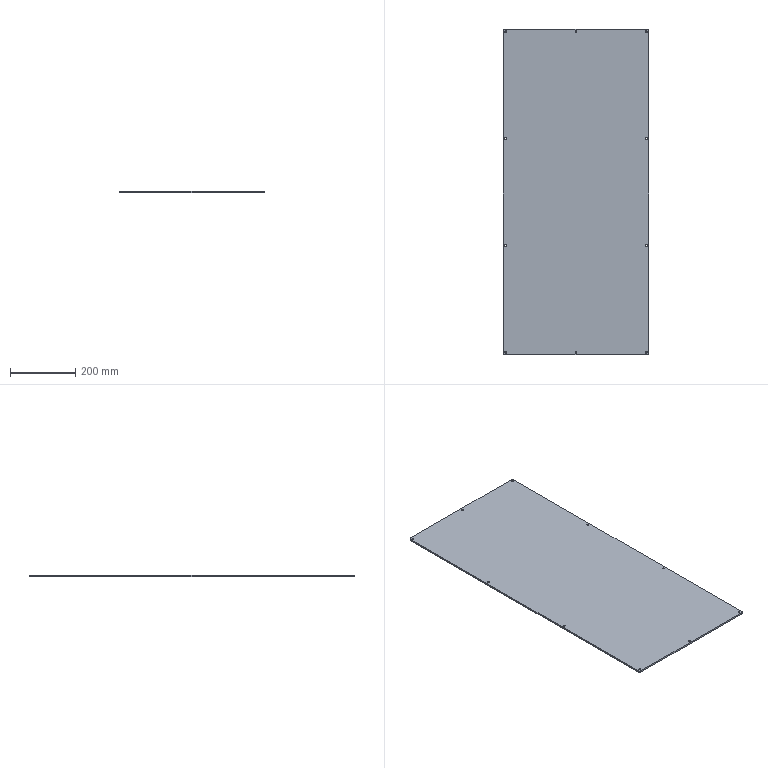Part | NX | features BREP 1 | 1 solid | 30 faces | box 446 x 996 x 5 mm | volume 2219652 mm3 | cylinder 24 | plane 6 | commonest cylinder face diameters 5.8 x20 10 x4
STEP:
#1=CARTESIAN_POINT('',(-218.,498.,5.));
#2=VERTEX_POINT('',#1);
#3=CARTESIAN_POINT('',(-223.,493.,5.));
#4=VERTEX_POINT('',#3);
#5=CARTESIAN_POINT('',(-218.,493.,5.));
#6=DIRECTION('',(0.,0.,1.));
#7=DIRECTION('',(1.,0.,0.));
#8=AXIS2_PLACEMENT_3D('',#5,#6,#7);
#9=CIRCLE('',#8,5.);
#10=EDGE_CURVE('',#2,#4,#9,.T.);
#11=ORIENTED_EDGE('',*,*,#10,.F.);
#12=CARTESIAN_POINT('',(-218.,498.,0.));
#13=VERTEX_POINT('',#12);
#14=CARTESIAN_POINT('',(-218.,498.,5.));
#15=DIRECTION('',(0.,0.,1.));
#16=VECTOR('',#15,1000.);
#17=LINE('',#14,#16);
#18=EDGE_CURVE('',#13,#2,#17,.T.);
#19=ORIENTED_EDGE('',*,*,#18,.F.);
#20=CARTESIAN_POINT('',(-223.,493.,0.));
#21=VERTEX_POINT('',#20);
#22=CARTESIAN_POINT('',(-218.,493.,0.));
#23=DIRECTION('',(0.,0.,-1.));
#24=DIRECTION('',(1.,0.,0.));
#25=AXIS2_PLACEMENT_3D('',#22,#23,#24);
#26=CIRCLE('',#25,5.);
#27=EDGE_CURVE('',#21,#13,#26,.T.);
#28=ORIENTED_EDGE('',*,*,#27,.F.);
#29=CARTESIAN_POINT('',(-223.,493.,5.));
#30=DIRECTION('',(0.,0.,-1.));
#31=VECTOR('',#30,1000.);
#32=LINE('',#29,#31);
#33=EDGE_CURVE('',#4,#21,#32,.T.);
#34=ORIENTED_EDGE('',*,*,#33,.F.);
#35=EDGE_LOOP('',(#11,#19,#28,#34));
#36=FACE_BOUND('',#35,.T.);
#37=CARTESIAN_POINT('',(-218.,493.,5.));
#38=DIRECTION('',(0.,0.,-1.));
#39=DIRECTION('',(-1.,0.,0.));
#40=AXIS2_PLACEMENT_3D('',#37,#38,#39);
#41=CYLINDRICAL_SURFACE('',#40,5.);
#42=ADVANCED_FACE('',(#36),#41,.T.);
#43=CARTESIAN_POINT('',(223.,493.,5.));
#44=VERTEX_POINT('',#43);
#45=CARTESIAN_POINT('',(218.,498.,5.));
#46=VERTEX_POINT('',#45);
#47=CARTESIAN_POINT('',(218.,493.,5.));
#48=DIRECTION('',(0.,0.,1.));
#49=DIRECTION('',(1.,0.,0.));
#50=AXIS2_PLACEMENT_3D('',#47,#48,#49);
#51=CIRCLE('',#50,5.);
#52=EDGE_CURVE('',#44,#46,#51,.T.);
#53=ORIENTED_EDGE('',*,*,#52,.F.);
#54=CARTESIAN_POINT('',(223.,493.,0.));
#55=VERTEX_POINT('',#54);
#56=CARTESIAN_POINT('',(223.,493.,5.));
#57=DIRECTION('',(0.,0.,1.));
#58=VECTOR('',#57,1000.);
#59=LINE('',#56,#58);
#60=EDGE_CURVE('',#55,#44,#59,.T.);
#61=ORIENTED_EDGE('',*,*,#60,.F.);
#62=CARTESIAN_POINT('',(218.,498.,0.));
#63=VERTEX_POINT('',#62);
#64=CARTESIAN_POINT('',(218.,493.,0.));
#65=DIRECTION('',(0.,0.,-1.));
#66=DIRECTION('',(1.,0.,0.));
#67=AXIS2_PLACEMENT_3D('',#64,#65,#66);
#68=CIRCLE('',#67,5.);
#69=EDGE_CURVE('',#63,#55,#68,.T.);
#70=ORIENTED_EDGE('',*,*,#69,.F.);
#71=CARTESIAN_POINT('',(218.,498.,5.));
#72=DIRECTION('',(0.,0.,-1.));
#73=VECTOR('',#72,1000.);
#74=LINE('',#71,#73);
#75=EDGE_CURVE('',#46,#63,#74,.T.);
#76=ORIENTED_EDGE('',*,*,#75,.F.);
#77=EDGE_LOOP('',(#53,#61,#70,#76));
#78=FACE_BOUND('',#77,.T.);
#79=CARTESIAN_POINT('',(218.,493.,5.));
#80=DIRECTION('',(0.,0.,-1.));
#81=DIRECTION('',(-1.,0.,0.));
#82=AXIS2_PLACEMENT_3D('',#79,#80,#81);
#83=CYLINDRICAL_SURFACE('',#82,5.);
#84=ADVANCED_FACE('',(#78),#83,.T.);
#85=CARTESIAN_POINT('',(218.,-498.,5.));
#86=VERTEX_POINT('',#85);
#87=CARTESIAN_POINT('',(223.,-493.,5.));
#88=VERTEX_POINT('',#87);
#89=CARTESIAN_POINT('',(218.,-493.,5.));
#90=DIRECTION('',(0.,0.,1.));
#91=DIRECTION('',(1.,0.,0.));
#92=AXIS2_PLACEMENT_3D('',#89,#90,#91);
#93=CIRCLE('',#92,5.);
#94=EDGE_CURVE('',#86,#88,#93,.T.);
#95=ORIENTED_EDGE('',*,*,#94,.F.);
#96=CARTESIAN_POINT('',(218.,-498.,0.));
#97=VERTEX_POINT('',#96);
#98=CARTESIAN_POINT('',(218.,-498.,5.));
#99=DIRECTION('',(0.,0.,1.));
#100=VECTOR('',#99,1000.);
#101=LINE('',#98,#100);
#102=EDGE_CURVE('',#97,#86,#101,.T.);
#103=ORIENTED_EDGE('',*,*,#102,.F.);
#104=CARTESIAN_POINT('',(223.,-493.,0.));
#105=VERTEX_POINT('',#104);
#106=CARTESIAN_POINT('',(218.,-493.,0.));
#107=DIRECTION('',(0.,0.,-1.));
#108=DIRECTION('',(1.,0.,0.));
#109=AXIS2_PLACEMENT_3D('',#106,#107,#108);
#110=CIRCLE('',#109,5.);
#111=EDGE_CURVE('',#105,#97,#110,.T.);
#112=ORIENTED_EDGE('',*,*,#111,.F.);
#113=CARTESIAN_POINT('',(223.,-493.,5.));
#114=DIRECTION('',(0.,0.,-1.));
#115=VECTOR('',#114,1000.);
#116=LINE('',#113,#115);
#117=EDGE_CURVE('',#88,#105,#116,.T.);
#118=ORIENTED_EDGE('',*,*,#117,.F.);
#119=EDGE_LOOP('',(#95,#103,#112,#118));
#120=FACE_BOUND('',#119,.T.);
#121=CARTESIAN_POINT('',(218.,-493.,5.));
#122=DIRECTION('',(0.,0.,-1.));
#123=DIRECTION('',(-1.,0.,0.));
#124=AXIS2_PLACEMENT_3D('',#121,#122,#123);
#125=CYLINDRICAL_SURFACE('',#124,5.);
#126=ADVANCED_FACE('',(#120),#125,.T.);
#127=CARTESIAN_POINT('',(-223.,-493.,5.));
#128=VERTEX_POINT('',#127);
#129=CARTESIAN_POINT('',(-218.,-498.,5.));
#130=VERTEX_POINT('',#129);
#131=CARTESIAN_POINT('',(-218.,-493.,5.));
#132=DIRECTION('',(0.,0.,1.));
#133=DIRECTION('',(1.,0.,0.));
#134=AXIS2_PLACEMENT_3D('',#131,#132,#133);
#135=CIRCLE('',#134,5.);
#136=EDGE_CURVE('',#128,#130,#135,.T.);
#137=ORIENTED_EDGE('',*,*,#136,.F.);
#138=CARTESIAN_POINT('',(-223.,-493.,0.));
#139=VERTEX_POINT('',#138);
#140=CARTESIAN_POINT('',(-223.,-493.,5.));
#141=DIRECTION('',(0.,0.,1.));
#142=VECTOR('',#141,1000.);
#143=LINE('',#140,#142);
#144=EDGE_CURVE('',#139,#128,#143,.T.);
#145=ORIENTED_EDGE('',*,*,#144,.F.);
#146=CARTESIAN_POINT('',(-218.,-498.,0.));
#147=VERTEX_POINT('',#146);
#148=CARTESIAN_POINT('',(-218.,-493.,0.));
#149=DIRECTION('',(0.,0.,-1.));
#150=DIRECTION('',(1.,0.,0.));
#151=AXIS2_PLACEMENT_3D('',#148,#149,#150);
#152=CIRCLE('',#151,5.);
#153=EDGE_CURVE('',#147,#139,#152,.T.);
#154=ORIENTED_EDGE('',*,*,#153,.F.);
#155=CARTESIAN_POINT('',(-218.,-498.,5.));
#156=DIRECTION('',(0.,0.,-1.));
#157=VECTOR('',#156,1000.);
#158=LINE('',#155,#157);
#159=EDGE_CURVE('',#130,#147,#158,.T.);
#160=ORIENTED_EDGE('',*,*,#159,.F.);
#161=EDGE_LOOP('',(#137,#145,#154,#160));
#162=FACE_BOUND('',#161,.T.);
#163=CARTESIAN_POINT('',(-218.,-493.,5.));
#164=DIRECTION('',(0.,0.,-1.));
#165=DIRECTION('',(-1.,0.,0.));
#166=AXIS2_PLACEMENT_3D('',#163,#164,#165);
#167=CYLINDRICAL_SURFACE('',#166,5.);
#168=ADVANCED_FACE('',(#162),#167,.T.);
#169=CARTESIAN_POINT('',(212.1,-490.,5.));
#170=VERTEX_POINT('',#169);
#171=CARTESIAN_POINT('',(212.1,-490.,0.));
#172=VERTEX_POINT('',#171);
#173=CARTESIAN_POINT('',(212.1,-490.,0.));
#174=DIRECTION('',(0.,0.,1.));
#175=VECTOR('',#174,1000.);
#176=LINE('',#173,#175);
#177=EDGE_CURVE('',#170,#172,#176,.F.);
#178=ORIENTED_EDGE('',*,*,#177,.T.);
#179=CARTESIAN_POINT('',(217.9,-490.,0.));
#180=VERTEX_POINT('',#179);
#181=CARTESIAN_POINT('',(215.,-490.,0.));
#182=DIRECTION('',(0.,0.,1.));
#183=DIRECTION('',(1.,0.,0.));
#184=AXIS2_PLACEMENT_3D('',#181,#182,#183);
#185=CIRCLE('',#184,2.9);
#186=EDGE_CURVE('',#180,#172,#185,.T.);
#187=ORIENTED_EDGE('',*,*,#186,.F.);
#188=CARTESIAN_POINT('',(217.9,-490.,5.));
#189=VERTEX_POINT('',#188);
#190=CARTESIAN_POINT('',(217.9,-490.,0.));
#191=DIRECTION('',(0.,0.,1.));
#192=VECTOR('',#191,1000.);
#193=LINE('',#190,#192);
#194=EDGE_CURVE('',#189,#180,#193,.F.);
#195=ORIENTED_EDGE('',*,*,#194,.F.);
#196=CARTESIAN_POINT('',(215.,-490.,5.));
#197=DIRECTION('',(0.,0.,1.));
#198=DIRECTION('',(1.,0.,0.));
#199=AXIS2_PLACEMENT_3D('',#196,#197,#198);
#200=CIRCLE('',#199,2.9);
#201=EDGE_CURVE('',#189,#170,#200,.T.);
#202=ORIENTED_EDGE('',*,*,#201,.T.);
#203=EDGE_LOOP('',(#178,#187,#195,#202));
#204=FACE_BOUND('',#203,.T.);
#205=CARTESIAN_POINT('',(215.,-490.,0.));
#206=DIRECTION('',(0.,0.,1.));
#207=DIRECTION('',(1.,0.,0.));
#208=AXIS2_PLACEMENT_3D('',#205,#206,#207);
#209=CYLINDRICAL_SURFACE('',#208,2.9);
#210=ADVANCED_FACE('',(#204),#209,.F.);
#211=CARTESIAN_POINT('',(212.1,163.333,5.));
#212=VERTEX_POINT('',#211);
#213=CARTESIAN_POINT('',(212.1,163.333,0.));
#214=VERTEX_POINT('',#213);
#215=CARTESIAN_POINT('',(212.1,163.333,0.));
#216=DIRECTION('',(0.,0.,1.));
#217=VECTOR('',#216,1000.);
#218=LINE('',#215,#217);
#219=EDGE_CURVE('',#212,#214,#218,.F.);
#220=ORIENTED_EDGE('',*,*,#219,.T.);
#221=CARTESIAN_POINT('',(217.9,163.333,0.));
#222=VERTEX_POINT('',#221);
#223=CARTESIAN_POINT('',(215.,163.333,0.));
#224=DIRECTION('',(0.,0.,1.));
#225=DIRECTION('',(1.,0.,0.));
#226=AXIS2_PLACEMENT_3D('',#223,#224,#225);
#227=CIRCLE('',#226,2.9);
#228=EDGE_CURVE('',#222,#214,#227,.T.);
#229=ORIENTED_EDGE('',*,*,#228,.F.);
#230=CARTESIAN_POINT('',(217.9,163.333,5.));
#231=VERTEX_POINT('',#230);
#232=CARTESIAN_POINT('',(217.9,163.333,0.));
#233=DIRECTION('',(0.,0.,1.));
#234=VECTOR('',#233,1000.);
#235=LINE('',#232,#234);
#236=EDGE_CURVE('',#231,#222,#235,.F.);
#237=ORIENTED_EDGE('',*,*,#236,.F.);
#238=CARTESIAN_POINT('',(215.,163.333,5.));
#239=DIRECTION('',(0.,0.,1.));
#240=DIRECTION('',(1.,0.,0.));
#241=AXIS2_PLACEMENT_3D('',#238,#239,#240);
#242=CIRCLE('',#241,2.9);
#243=EDGE_CURVE('',#231,#212,#242,.T.);
#244=ORIENTED_EDGE('',*,*,#243,.T.);
#245=EDGE_LOOP('',(#220,#229,#237,#244));
#246=FACE_BOUND('',#245,.T.);
#247=CARTESIAN_POINT('',(215.,163.333,0.));
#248=DIRECTION('',(0.,0.,1.));
#249=DIRECTION('',(1.,0.,0.));
#250=AXIS2_PLACEMENT_3D('',#247,#248,#249);
#251=CYLINDRICAL_SURFACE('',#250,2.9);
#252=ADVANCED_FACE('',(#246),#251,.F.);
#253=CARTESIAN_POINT('',(212.1,-163.333,5.));
#254=VERTEX_POINT('',#253);
#255=CARTESIAN_POINT('',(212.1,-163.333,0.));
#256=VERTEX_POINT('',#255);
#257=CARTESIAN_POINT('',(212.1,-163.333,0.));
#258=DIRECTION('',(0.,0.,1.));
#259=VECTOR('',#258,1000.);
#260=LINE('',#257,#259);
#261=EDGE_CURVE('',#254,#256,#260,.F.);
#262=ORIENTED_EDGE('',*,*,#261,.T.);
#263=CARTESIAN_POINT('',(217.9,-163.333,0.));
#264=VERTEX_POINT('',#263);
#265=CARTESIAN_POINT('',(215.,-163.333,0.));
#266=DIRECTION('',(0.,0.,1.));
#267=DIRECTION('',(1.,0.,0.));
#268=AXIS2_PLACEMENT_3D('',#265,#266,#267);
#269=CIRCLE('',#268,2.9);
#270=EDGE_CURVE('',#264,#256,#269,.T.);
#271=ORIENTED_EDGE('',*,*,#270,.F.);
#272=CARTESIAN_POINT('',(217.9,-163.333,5.));
#273=VERTEX_POINT('',#272);
#274=CARTESIAN_POINT('',(217.9,-163.333,0.));
#275=DIRECTION('',(0.,0.,1.));
#276=VECTOR('',#275,1000.);
#277=LINE('',#274,#276);
#278=EDGE_CURVE('',#273,#264,#277,.F.);
#279=ORIENTED_EDGE('',*,*,#278,.F.);
#280=CARTESIAN_POINT('',(215.,-163.333,5.));
#281=DIRECTION('',(0.,0.,1.));
#282=DIRECTION('',(1.,0.,0.));
#283=AXIS2_PLACEMENT_3D('',#280,#281,#282);
#284=CIRCLE('',#283,2.9);
#285=EDGE_CURVE('',#273,#254,#284,.T.);
#286=ORIENTED_EDGE('',*,*,#285,.T.);
#287=EDGE_LOOP('',(#262,#271,#279,#286));
#288=FACE_BOUND('',#287,.T.);
#289=CARTESIAN_POINT('',(215.,-163.333,0.));
#290=DIRECTION('',(0.,0.,1.));
#291=DIRECTION('',(1.,0.,0.));
#292=AXIS2_PLACEMENT_3D('',#289,#290,#291);
#293=CYLINDRICAL_SURFACE('',#292,2.9);
#294=ADVANCED_FACE('',(#288),#293,.F.);
#295=CARTESIAN_POINT('',(-217.9,163.333,5.));
#296=VERTEX_POINT('',#295);
#297=CARTESIAN_POINT('',(-217.9,163.333,0.));
#298=VERTEX_POINT('',#297);
#299=CARTESIAN_POINT('',(-217.9,163.333,0.));
#300=DIRECTION('',(0.,0.,1.));
#301=VECTOR('',#300,1000.);
#302=LINE('',#299,#301);
#303=EDGE_CURVE('',#296,#298,#302,.F.);
#304=ORIENTED_EDGE('',*,*,#303,.T.);
#305=CARTESIAN_POINT('',(-212.1,163.333,0.));
#306=VERTEX_POINT('',#305);
#307=CARTESIAN_POINT('',(-215.,163.333,0.));
#308=DIRECTION('',(0.,0.,1.));
#309=DIRECTION('',(1.,0.,0.));
#310=AXIS2_PLACEMENT_3D('',#307,#308,#309);
#311=CIRCLE('',#310,2.9);
#312=EDGE_CURVE('',#306,#298,#311,.T.);
#313=ORIENTED_EDGE('',*,*,#312,.F.);
#314=CARTESIAN_POINT('',(-212.1,163.333,5.));
#315=VERTEX_POINT('',#314);
#316=CARTESIAN_POINT('',(-212.1,163.333,0.));
#317=DIRECTION('',(0.,0.,1.));
#318=VECTOR('',#317,1000.);
#319=LINE('',#316,#318);
#320=EDGE_CURVE('',#315,#306,#319,.F.);
#321=ORIENTED_EDGE('',*,*,#320,.F.);
#322=CARTESIAN_POINT('',(-215.,163.333,5.));
#323=DIRECTION('',(0.,0.,1.));
#324=DIRECTION('',(1.,0.,0.));
#325=AXIS2_PLACEMENT_3D('',#322,#323,#324);
#326=CIRCLE('',#325,2.9);
#327=EDGE_CURVE('',#315,#296,#326,.T.);
#328=ORIENTED_EDGE('',*,*,#327,.T.);
#329=EDGE_LOOP('',(#304,#313,#321,#328));
#330=FACE_BOUND('',#329,.T.);
#331=CARTESIAN_POINT('',(-215.,163.333,0.));
#332=DIRECTION('',(0.,0.,1.));
#333=DIRECTION('',(1.,0.,0.));
#334=AXIS2_PLACEMENT_3D('',#331,#332,#333);
#335=CYLINDRICAL_SURFACE('',#334,2.9);
#336=ADVANCED_FACE('',(#330),#335,.F.);
#337=CARTESIAN_POINT('',(-2.9,-490.,5.));
#338=VERTEX_POINT('',#337);
#339=CARTESIAN_POINT('',(-2.9,-490.,0.));
#340=VERTEX_POINT('',#339);
#341=CARTESIAN_POINT('',(-2.9,-490.,0.));
#342=DIRECTION('',(0.,0.,1.));
#343=VECTOR('',#342,1000.);
#344=LINE('',#341,#343);
#345=EDGE_CURVE('',#338,#340,#344,.F.);
#346=ORIENTED_EDGE('',*,*,#345,.T.);
#347=CARTESIAN_POINT('',(2.9,-490.,0.));
#348=VERTEX_POINT('',#347);
#349=CARTESIAN_POINT('',(0.,-490.,0.));
#350=DIRECTION('',(0.,0.,1.));
#351=DIRECTION('',(1.,0.,0.));
#352=AXIS2_PLACEMENT_3D('',#349,#350,#351);
#353=CIRCLE('',#352,2.9);
#354=EDGE_CURVE('',#348,#340,#353,.T.);
#355=ORIENTED_EDGE('',*,*,#354,.F.);
#356=CARTESIAN_POINT('',(2.9,-490.,5.));
#357=VERTEX_POINT('',#356);
#358=CARTESIAN_POINT('',(2.9,-490.,0.));
#359=DIRECTION('',(0.,0.,1.));
#360=VECTOR('',#359,1000.);
#361=LINE('',#358,#360);
#362=EDGE_CURVE('',#357,#348,#361,.F.);
#363=ORIENTED_EDGE('',*,*,#362,.F.);
#364=CARTESIAN_POINT('',(0.,-490.,5.));
#365=DIRECTION('',(0.,0.,1.));
#366=DIRECTION('',(1.,0.,0.));
#367=AXIS2_PLACEMENT_3D('',#364,#365,#366);
#368=CIRCLE('',#367,2.9);
#369=EDGE_CURVE('',#357,#338,#368,.T.);
#370=ORIENTED_EDGE('',*,*,#369,.T.);
#371=EDGE_LOOP('',(#346,#355,#363,#370));
#372=FACE_BOUND('',#371,.T.);
#373=CARTESIAN_POINT('',(0.,-490.,0.));
#374=DIRECTION('',(0.,0.,1.));
#375=DIRECTION('',(1.,0.,0.));
#376=AXIS2_PLACEMENT_3D('',#373,#374,#375);
#377=CYLINDRICAL_SURFACE('',#376,2.9);
#378=ADVANCED_FACE('',(#372),#377,.F.);
#379=CARTESIAN_POINT('',(-217.9,-490.,5.));
#380=VERTEX_POINT('',#379);
#381=CARTESIAN_POINT('',(-217.9,-490.,0.));
#382=VERTEX_POINT('',#381);
#383=CARTESIAN_POINT('',(-217.9,-490.,0.));
#384=DIRECTION('',(0.,0.,1.));
#385=VECTOR('',#384,1000.);
#386=LINE('',#383,#385);
#387=EDGE_CURVE('',#380,#382,#386,.F.);
#388=ORIENTED_EDGE('',*,*,#387,.T.);
#389=CARTESIAN_POINT('',(-212.1,-490.,0.));
#390=VERTEX_POINT('',#389);
#391=CARTESIAN_POINT('',(-215.,-490.,0.));
#392=DIRECTION('',(0.,0.,1.));
#393=DIRECTION('',(1.,0.,0.));
#394=AXIS2_PLACEMENT_3D('',#391,#392,#393);
#395=CIRCLE('',#394,2.9);
#396=EDGE_CURVE('',#390,#382,#395,.T.);
#397=ORIENTED_EDGE('',*,*,#396,.F.);
#398=CARTESIAN_POINT('',(-212.1,-490.,5.));
#399=VERTEX_POINT('',#398);
#400=CARTESIAN_POINT('',(-212.1,-490.,0.));
#401=DIRECTION('',(0.,0.,1.));
#402=VECTOR('',#401,1000.);
#403=LINE('',#400,#402);
#404=EDGE_CURVE('',#399,#390,#403,.F.);
#405=ORIENTED_EDGE('',*,*,#404,.F.);
#406=CARTESIAN_POINT('',(-215.,-490.,5.));
#407=DIRECTION('',(0.,0.,1.));
#408=DIRECTION('',(1.,0.,0.));
#409=AXIS2_PLACEMENT_3D('',#406,#407,#408);
#410=CIRCLE('',#409,2.9);
#411=EDGE_CURVE('',#399,#380,#410,.T.);
#412=ORIENTED_EDGE('',*,*,#411,.T.);
#413=EDGE_LOOP('',(#388,#397,#405,#412));
#414=FACE_BOUND('',#413,.T.);
#415=CARTESIAN_POINT('',(-215.,-490.,0.));
#416=DIRECTION('',(0.,0.,1.));
#417=DIRECTION('',(1.,0.,0.));
#418=AXIS2_PLACEMENT_3D('',#415,#416,#417);
#419=CYLINDRICAL_SURFACE('',#418,2.9);
#420=ADVANCED_FACE('',(#414),#419,.F.);
#421=CARTESIAN_POINT('',(212.1,490.,5.));
#422=VERTEX_POINT('',#421);
#423=CARTESIAN_POINT('',(212.1,490.,0.));
#424=VERTEX_POINT('',#423);
#425=CARTESIAN_POINT('',(212.1,490.,0.));
#426=DIRECTION('',(0.,0.,1.));
#427=VECTOR('',#426,1000.);
#428=LINE('',#425,#427);
#429=EDGE_CURVE('',#422,#424,#428,.F.);
#430=ORIENTED_EDGE('',*,*,#429,.T.);
#431=CARTESIAN_POINT('',(217.9,490.,0.));
#432=VERTEX_POINT('',#431);
#433=CARTESIAN_POINT('',(215.,490.,0.));
#434=DIRECTION('',(0.,0.,1.));
#435=DIRECTION('',(1.,0.,0.));
#436=AXIS2_PLACEMENT_3D('',#433,#434,#435);
#437=CIRCLE('',#436,2.9);
#438=EDGE_CURVE('',#432,#424,#437,.T.);
#439=ORIENTED_EDGE('',*,*,#438,.F.);
#440=CARTESIAN_POINT('',(217.9,490.,5.));
#441=VERTEX_POINT('',#440);
#442=CARTESIAN_POINT('',(217.9,490.,0.));
#443=DIRECTION('',(0.,0.,1.));
#444=VECTOR('',#443,1000.);
#445=LINE('',#442,#444);
#446=EDGE_CURVE('',#441,#432,#445,.F.);
#447=ORIENTED_EDGE('',*,*,#446,.F.);
#448=CARTESIAN_POINT('',(215.,490.,5.));
#449=DIRECTION('',(0.,0.,1.));
#450=DIRECTION('',(1.,0.,0.));
#451=AXIS2_PLACEMENT_3D('',#448,#449,#450);
#452=CIRCLE('',#451,2.9);
#453=EDGE_CURVE('',#441,#422,#452,.T.);
#454=ORIENTED_EDGE('',*,*,#453,.T.);
#455=EDGE_LOOP('',(#430,#439,#447,#454));
#456=FACE_BOUND('',#455,.T.);
#457=CARTESIAN_POINT('',(215.,490.,0.));
#458=DIRECTION('',(0.,0.,1.));
#459=DIRECTION('',(1.,0.,0.));
#460=AXIS2_PLACEMENT_3D('',#457,#458,#459);
#461=CYLINDRICAL_SURFACE('',#460,2.9);
#462=ADVANCED_FACE('',(#456),#461,.F.);
#463=CARTESIAN_POINT('',(-2.9,490.,5.));
#464=VERTEX_POINT('',#463);
#465=CARTESIAN_POINT('',(-2.9,490.,0.));
#466=VERTEX_POINT('',#465);
#467=CARTESIAN_POINT('',(-2.9,490.,0.));
#468=DIRECTION('',(0.,0.,1.));
#469=VECTOR('',#468,1000.);
#470=LINE('',#467,#469);
#471=EDGE_CURVE('',#464,#466,#470,.F.);
#472=ORIENTED_EDGE('',*,*,#471,.T.);
#473=CARTESIAN_POINT('',(2.9,490.,0.));
#474=VERTEX_POINT('',#473);
#475=CARTESIAN_POINT('',(0.,490.,0.));
#476=DIRECTION('',(0.,0.,1.));
#477=DIRECTION('',(1.,0.,0.));
#478=AXIS2_PLACEMENT_3D('',#475,#476,#477);
#479=CIRCLE('',#478,2.9);
#480=EDGE_CURVE('',#474,#466,#479,.T.);
#481=ORIENTED_EDGE('',*,*,#480,.F.);
#482=CARTESIAN_POINT('',(2.9,490.,5.));
#483=VERTEX_POINT('',#482);
#484=CARTESIAN_POINT('',(2.9,490.,0.));
#485=DIRECTION('',(0.,0.,1.));
#486=VECTOR('',#485,1000.);
#487=LINE('',#484,#486);
#488=EDGE_CURVE('',#483,#474,#487,.F.);
#489=ORIENTED_EDGE('',*,*,#488,.F.);
#490=CARTESIAN_POINT('',(0.,490.,5.));
#491=DIRECTION('',(0.,0.,1.));
#492=DIRECTION('',(1.,0.,0.));
#493=AXIS2_PLACEMENT_3D('',#490,#491,#492);
#494=CIRCLE('',#493,2.9);
#495=EDGE_CURVE('',#483,#464,#494,.T.);
#496=ORIENTED_EDGE('',*,*,#495,.T.);
#497=EDGE_LOOP('',(#472,#481,#489,#496));
#498=FACE_BOUND('',#497,.T.);
#499=CARTESIAN_POINT('',(0.,490.,0.));
#500=DIRECTION('',(0.,0.,1.));
#501=DIRECTION('',(1.,0.,0.));
#502=AXIS2_PLACEMENT_3D('',#499,#500,#501);
#503=CYLINDRICAL_SURFACE('',#502,2.9);
#504=ADVANCED_FACE('',(#498),#503,.F.);
#505=CARTESIAN_POINT('',(-217.9,-163.333,5.));
#506=VERTEX_POINT('',#505);
#507=CARTESIAN_POINT('',(-217.9,-163.333,0.));
#508=VERTEX_POINT('',#507);
#509=CARTESIAN_POINT('',(-217.9,-163.333,0.));
#510=DIRECTION('',(0.,0.,1.));
#511=VECTOR('',#510,1000.);
#512=LINE('',#509,#511);
#513=EDGE_CURVE('',#506,#508,#512,.F.);
#514=ORIENTED_EDGE('',*,*,#513,.T.);
#515=CARTESIAN_POINT('',(-212.1,-163.333,0.));
#516=VERTEX_POINT('',#515);
#517=CARTESIAN_POINT('',(-215.,-163.333,0.));
#518=DIRECTION('',(0.,0.,1.));
#519=DIRECTION('',(1.,0.,0.));
#520=AXIS2_PLACEMENT_3D('',#517,#518,#519);
#521=CIRCLE('',#520,2.9);
#522=EDGE_CURVE('',#516,#508,#521,.T.);
#523=ORIENTED_EDGE('',*,*,#522,.F.);
#524=CARTESIAN_POINT('',(-212.1,-163.333,5.));
#525=VERTEX_POINT('',#524);
#526=CARTESIAN_POINT('',(-212.1,-163.333,0.));
#527=DIRECTION('',(0.,0.,1.));
#528=VECTOR('',#527,1000.);
#529=LINE('',#526,#528);
#530=EDGE_CURVE('',#525,#516,#529,.F.);
#531=ORIENTED_EDGE('',*,*,#530,.F.);
#532=CARTESIAN_POINT('',(-215.,-163.333,5.));
#533=DIRECTION('',(0.,0.,1.));
#534=DIRECTION('',(1.,0.,0.));
#535=AXIS2_PLACEMENT_3D('',#532,#533,#534);
#536=CIRCLE('',#535,2.9);
#537=EDGE_CURVE('',#525,#506,#536,.T.);
#538=ORIENTED_EDGE('',*,*,#537,.T.);
#539=EDGE_LOOP('',(#514,#523,#531,#538));
#540=FACE_BOUND('',#539,.T.);
#541=CARTESIAN_POINT('',(-215.,-163.333,0.));
#542=DIRECTION('',(0.,0.,1.));
#543=DIRECTION('',(1.,0.,0.));
#544=AXIS2_PLACEMENT_3D('',#541,#542,#543);
#545=CYLINDRICAL_SURFACE('',#544,2.9);
#546=ADVANCED_FACE('',(#540),#545,.F.);
#547=CARTESIAN_POINT('',(-217.9,490.,5.));
#548=VERTEX_POINT('',#547);
#549=CARTESIAN_POINT('',(-217.9,490.,0.));
#550=VERTEX_POINT('',#549);
#551=CARTESIAN_POINT('',(-217.9,490.,0.));
#552=DIRECTION('',(0.,0.,1.));
#553=VECTOR('',#552,1000.);
#554=LINE('',#551,#553);
#555=EDGE_CURVE('',#548,#550,#554,.F.);
#556=ORIENTED_EDGE('',*,*,#555,.T.);
#557=CARTESIAN_POINT('',(-212.1,490.,0.));
#558=VERTEX_POINT('',#557);
#559=CARTESIAN_POINT('',(-215.,490.,0.));
#560=DIRECTION('',(0.,0.,1.));
#561=DIRECTION('',(1.,0.,0.));
#562=AXIS2_PLACEMENT_3D('',#559,#560,#561);
#563=CIRCLE('',#562,2.9);
#564=EDGE_CURVE('',#558,#550,#563,.T.);
#565=ORIENTED_EDGE('',*,*,#564,.F.);
#566=CARTESIAN_POINT('',(-212.1,490.,5.));
#567=VERTEX_POINT('',#566);
#568=CARTESIAN_POINT('',(-212.1,490.,0.));
#569=DIRECTION('',(0.,0.,1.));
#570=VECTOR('',#569,1000.);
#571=LINE('',#568,#570);
#572=EDGE_CURVE('',#567,#558,#571,.F.);
#573=ORIENTED_EDGE('',*,*,#572,.F.);
#574=CARTESIAN_POINT('',(-215.,490.,5.));
#575=DIRECTION('',(0.,0.,1.));
#576=DIRECTION('',(1.,0.,0.));
#577=AXIS2_PLACEMENT_3D('',#574,#575,#576);
#578=CIRCLE('',#577,2.9);
#579=EDGE_CURVE('',#567,#548,#578,.T.);
#580=ORIENTED_EDGE('',*,*,#579,.T.);
#581=EDGE_LOOP('',(#556,#565,#573,#580));
#582=FACE_BOUND('',#581,.T.);
#583=CARTESIAN_POINT('',(-215.,490.,0.));
#584=DIRECTION('',(0.,0.,1.));
#585=DIRECTION('',(1.,0.,0.));
#586=AXIS2_PLACEMENT_3D('',#583,#584,#585);
#587=CYLINDRICAL_SURFACE('',#586,2.9);
#588=ADVANCED_FACE('',(#582),#587,.F.);
#589=CARTESIAN_POINT('',(223.,-498.,0.));
#590=DIRECTION('',(1.,0.,0.));
#591=VECTOR('',#590,1000.);
#592=LINE('',#589,#591);
#593=EDGE_CURVE('',#147,#97,#592,.T.);
#594=ORIENTED_EDGE('',*,*,#593,.F.);
#595=ORIENTED_EDGE('',*,*,#153,.T.);
#596=CARTESIAN_POINT('',(-223.,-498.,0.));
#597=DIRECTION('',(0.,-1.,0.));
#598=VECTOR('',#597,1000.);
#599=LINE('',#596,#598);
#600=EDGE_CURVE('',#21,#139,#599,.T.);
#601=ORIENTED_EDGE('',*,*,#600,.F.);
#602=ORIENTED_EDGE('',*,*,#27,.T.);
#603=CARTESIAN_POINT('',(223.,498.,0.));
#604=DIRECTION('',(-1.,0.,0.));
#605=VECTOR('',#604,1000.);
#606=LINE('',#603,#605);
#607=EDGE_CURVE('',#63,#13,#606,.T.);
#608=ORIENTED_EDGE('',*,*,#607,.F.);
#609=ORIENTED_EDGE('',*,*,#69,.T.);
#610=CARTESIAN_POINT('',(223.,-498.,0.));
#611=DIRECTION('',(0.,1.,0.));
#612=VECTOR('',#611,1000.);
#613=LINE('',#610,#612);
#614=EDGE_CURVE('',#105,#55,#613,.T.);
#615=ORIENTED_EDGE('',*,*,#614,.F.);
#616=ORIENTED_EDGE('',*,*,#111,.T.);
#617=EDGE_LOOP('',(#594,#595,#601,#602,#608,#609,#615,#616));
#618=FACE_BOUND('',#617,.T.);
#619=ORIENTED_EDGE('',*,*,#564,.T.);
#620=CARTESIAN_POINT('',(-215.,490.,0.));
#621=DIRECTION('',(0.,0.,1.));
#622=DIRECTION('',(1.,0.,0.));
#623=AXIS2_PLACEMENT_3D('',#620,#621,#622);
#624=CIRCLE('',#623,2.9);
#625=EDGE_CURVE('',#550,#558,#624,.T.);
#626=ORIENTED_EDGE('',*,*,#625,.T.);
#627=EDGE_LOOP('',(#619,#626));
#628=FACE_BOUND('',#627,.T.);
#629=ORIENTED_EDGE('',*,*,#522,.T.);
#630=CARTESIAN_POINT('',(-215.,-163.333,0.));
#631=DIRECTION('',(0.,0.,1.));
#632=DIRECTION('',(1.,0.,0.));
#633=AXIS2_PLACEMENT_3D('',#630,#631,#632);
#634=CIRCLE('',#633,2.9);
#635=EDGE_CURVE('',#508,#516,#634,.T.);
#636=ORIENTED_EDGE('',*,*,#635,.T.);
#637=EDGE_LOOP('',(#629,#636));
#638=FACE_BOUND('',#637,.T.);
#639=ORIENTED_EDGE('',*,*,#480,.T.);
#640=CARTESIAN_POINT('',(0.,490.,0.));
#641=DIRECTION('',(0.,0.,1.));
#642=DIRECTION('',(1.,0.,0.));
#643=AXIS2_PLACEMENT_3D('',#640,#641,#642);
#644=CIRCLE('',#643,2.9);
#645=EDGE_CURVE('',#466,#474,#644,.T.);
#646=ORIENTED_EDGE('',*,*,#645,.T.);
#647=EDGE_LOOP('',(#639,#646));
#648=FACE_BOUND('',#647,.T.);
#649=ORIENTED_EDGE('',*,*,#438,.T.);
#650=CARTESIAN_POINT('',(215.,490.,0.));
#651=DIRECTION('',(0.,0.,1.));
#652=DIRECTION('',(1.,0.,0.));
#653=AXIS2_PLACEMENT_3D('',#650,#651,#652);
#654=CIRCLE('',#653,2.9);
#655=EDGE_CURVE('',#424,#432,#654,.T.);
#656=ORIENTED_EDGE('',*,*,#655,.T.);
#657=EDGE_LOOP('',(#649,#656));
#658=FACE_BOUND('',#657,.T.);
#659=ORIENTED_EDGE('',*,*,#396,.T.);
#660=CARTESIAN_POINT('',(-215.,-490.,0.));
#661=DIRECTION('',(0.,0.,1.));
#662=DIRECTION('',(1.,0.,0.));
#663=AXIS2_PLACEMENT_3D('',#660,#661,#662);
#664=CIRCLE('',#663,2.9);
#665=EDGE_CURVE('',#382,#390,#664,.T.);
#666=ORIENTED_EDGE('',*,*,#665,.T.);
#667=EDGE_LOOP('',(#659,#666));
#668=FACE_BOUND('',#667,.T.);
#669=ORIENTED_EDGE('',*,*,#354,.T.);
#670=CARTESIAN_POINT('',(0.,-490.,0.));
#671=DIRECTION('',(0.,0.,1.));
#672=DIRECTION('',(1.,0.,0.));
#673=AXIS2_PLACEMENT_3D('',#670,#671,#672);
#674=CIRCLE('',#673,2.9);
#675=EDGE_CURVE('',#340,#348,#674,.T.);
#676=ORIENTED_EDGE('',*,*,#675,.T.);
#677=EDGE_LOOP('',(#669,#676));
#678=FACE_BOUND('',#677,.T.);
#679=ORIENTED_EDGE('',*,*,#312,.T.);
#680=CARTESIAN_POINT('',(-215.,163.333,0.));
#681=DIRECTION('',(0.,0.,1.));
#682=DIRECTION('',(1.,0.,0.));
#683=AXIS2_PLACEMENT_3D('',#680,#681,#682);
#684=CIRCLE('',#683,2.9);
#685=EDGE_CURVE('',#298,#306,#684,.T.);
#686=ORIENTED_EDGE('',*,*,#685,.T.);
#687=EDGE_LOOP('',(#679,#686));
#688=FACE_BOUND('',#687,.T.);
#689=ORIENTED_EDGE('',*,*,#270,.T.);
#690=CARTESIAN_POINT('',(215.,-163.333,0.));
#691=DIRECTION('',(0.,0.,1.));
#692=DIRECTION('',(1.,0.,0.));
#693=AXIS2_PLACEMENT_3D('',#690,#691,#692);
#694=CIRCLE('',#693,2.9);
#695=EDGE_CURVE('',#256,#264,#694,.T.);
#696=ORIENTED_EDGE('',*,*,#695,.T.);
#697=EDGE_LOOP('',(#689,#696));
#698=FACE_BOUND('',#697,.T.);
#699=ORIENTED_EDGE('',*,*,#228,.T.);
#700=CARTESIAN_POINT('',(215.,163.333,0.));
#701=DIRECTION('',(0.,0.,1.));
#702=DIRECTION('',(1.,0.,0.));
#703=AXIS2_PLACEMENT_3D('',#700,#701,#702);
#704=CIRCLE('',#703,2.9);
#705=EDGE_CURVE('',#214,#222,#704,.T.);
#706=ORIENTED_EDGE('',*,*,#705,.T.);
#707=EDGE_LOOP('',(#699,#706));
#708=FACE_BOUND('',#707,.T.);
#709=ORIENTED_EDGE('',*,*,#186,.T.);
#710=CARTESIAN_POINT('',(215.,-490.,0.));
#711=DIRECTION('',(0.,0.,1.));
#712=DIRECTION('',(1.,0.,0.));
#713=AXIS2_PLACEMENT_3D('',#710,#711,#712);
#714=CIRCLE('',#713,2.9);
#715=EDGE_CURVE('',#172,#180,#714,.T.);
#716=ORIENTED_EDGE('',*,*,#715,.T.);
#717=EDGE_LOOP('',(#709,#716));
#718=FACE_BOUND('',#717,.T.);
#719=CARTESIAN_POINT('',(0.,0.,0.));
#720=DIRECTION('',(0.,0.,1.));
#721=DIRECTION('',(1.,0.,0.));
#722=AXIS2_PLACEMENT_3D('',#719,#720,#721);
#723=PLANE('',#722);
#724=ADVANCED_FACE('',(#618,#628,#638,#648,#658,#668,#678,#688,#698,#708,#718),#723,.F.);
#725=CARTESIAN_POINT('',(-223.,-498.,5.));
#726=DIRECTION('',(0.,-1.,0.));
#727=VECTOR('',#726,1000.);
#728=LINE('',#725,#727);
#729=EDGE_CURVE('',#4,#128,#728,.T.);
#730=ORIENTED_EDGE('',*,*,#729,.T.);
#731=ORIENTED_EDGE('',*,*,#136,.T.);
#732=CARTESIAN_POINT('',(223.,-498.,5.));
#733=DIRECTION('',(1.,0.,0.));
#734=VECTOR('',#733,1000.);
#735=LINE('',#732,#734);
#736=EDGE_CURVE('',#130,#86,#735,.T.);
#737=ORIENTED_EDGE('',*,*,#736,.T.);
#738=ORIENTED_EDGE('',*,*,#94,.T.);
#739=CARTESIAN_POINT('',(223.,-498.,5.));
#740=DIRECTION('',(0.,1.,0.));
#741=VECTOR('',#740,1000.);
#742=LINE('',#739,#741);
#743=EDGE_CURVE('',#88,#44,#742,.T.);
#744=ORIENTED_EDGE('',*,*,#743,.T.);
#745=ORIENTED_EDGE('',*,*,#52,.T.);
#746=CARTESIAN_POINT('',(223.,498.,5.));
#747=DIRECTION('',(-1.,0.,0.));
#748=VECTOR('',#747,1000.);
#749=LINE('',#746,#748);
#750=EDGE_CURVE('',#46,#2,#749,.T.);
#751=ORIENTED_EDGE('',*,*,#750,.T.);
#752=ORIENTED_EDGE('',*,*,#10,.T.);
#753=EDGE_LOOP('',(#730,#731,#737,#738,#744,#745,#751,#752));
#754=FACE_BOUND('',#753,.T.);
#755=ORIENTED_EDGE('',*,*,#579,.F.);
#756=CARTESIAN_POINT('',(-215.,490.,5.));
#757=DIRECTION('',(0.,0.,1.));
#758=DIRECTION('',(1.,0.,0.));
#759=AXIS2_PLACEMENT_3D('',#756,#757,#758);
#760=CIRCLE('',#759,2.9);
#761=EDGE_CURVE('',#548,#567,#760,.T.);
#762=ORIENTED_EDGE('',*,*,#761,.F.);
#763=EDGE_LOOP('',(#755,#762));
#764=FACE_BOUND('',#763,.T.);
#765=ORIENTED_EDGE('',*,*,#537,.F.);
#766=CARTESIAN_POINT('',(-215.,-163.333,5.));
#767=DIRECTION('',(0.,0.,1.));
#768=DIRECTION('',(1.,0.,0.));
#769=AXIS2_PLACEMENT_3D('',#766,#767,#768);
#770=CIRCLE('',#769,2.9);
#771=EDGE_CURVE('',#506,#525,#770,.T.);
#772=ORIENTED_EDGE('',*,*,#771,.F.);
#773=EDGE_LOOP('',(#765,#772));
#774=FACE_BOUND('',#773,.T.);
#775=ORIENTED_EDGE('',*,*,#495,.F.);
#776=CARTESIAN_POINT('',(0.,490.,5.));
#777=DIRECTION('',(0.,0.,1.));
#778=DIRECTION('',(1.,0.,0.));
#779=AXIS2_PLACEMENT_3D('',#776,#777,#778);
#780=CIRCLE('',#779,2.9);
#781=EDGE_CURVE('',#464,#483,#780,.T.);
#782=ORIENTED_EDGE('',*,*,#781,.F.);
#783=EDGE_LOOP('',(#775,#782));
#784=FACE_BOUND('',#783,.T.);
#785=ORIENTED_EDGE('',*,*,#453,.F.);
#786=CARTESIAN_POINT('',(215.,490.,5.));
#787=DIRECTION('',(0.,0.,1.));
#788=DIRECTION('',(1.,0.,0.));
#789=AXIS2_PLACEMENT_3D('',#786,#787,#788);
#790=CIRCLE('',#789,2.9);
#791=EDGE_CURVE('',#422,#441,#790,.T.);
#792=ORIENTED_EDGE('',*,*,#791,.F.);
#793=EDGE_LOOP('',(#785,#792));
#794=FACE_BOUND('',#793,.T.);
#795=ORIENTED_EDGE('',*,*,#411,.F.);
#796=CARTESIAN_POINT('',(-215.,-490.,5.));
#797=DIRECTION('',(0.,0.,1.));
#798=DIRECTION('',(1.,0.,0.));
#799=AXIS2_PLACEMENT_3D('',#796,#797,#798);
#800=CIRCLE('',#799,2.9);
#801=EDGE_CURVE('',#380,#399,#800,.T.);
#802=ORIENTED_EDGE('',*,*,#801,.F.);
#803=EDGE_LOOP('',(#795,#802));
#804=FACE_BOUND('',#803,.T.);
#805=ORIENTED_EDGE('',*,*,#369,.F.);
#806=CARTESIAN_POINT('',(0.,-490.,5.));
#807=DIRECTION('',(0.,0.,1.));
#808=DIRECTION('',(1.,0.,0.));
#809=AXIS2_PLACEMENT_3D('',#806,#807,#808);
#810=CIRCLE('',#809,2.9);
#811=EDGE_CURVE('',#338,#357,#810,.T.);
#812=ORIENTED_EDGE('',*,*,#811,.F.);
#813=EDGE_LOOP('',(#805,#812));
#814=FACE_BOUND('',#813,.T.);
#815=ORIENTED_EDGE('',*,*,#327,.F.);
#816=CARTESIAN_POINT('',(-215.,163.333,5.));
#817=DIRECTION('',(0.,0.,1.));
#818=DIRECTION('',(1.,0.,0.));
#819=AXIS2_PLACEMENT_3D('',#816,#817,#818);
#820=CIRCLE('',#819,2.9);
#821=EDGE_CURVE('',#296,#315,#820,.T.);
#822=ORIENTED_EDGE('',*,*,#821,.F.);
#823=EDGE_LOOP('',(#815,#822));
#824=FACE_BOUND('',#823,.T.);
#825=ORIENTED_EDGE('',*,*,#285,.F.);
#826=CARTESIAN_POINT('',(215.,-163.333,5.));
#827=DIRECTION('',(0.,0.,1.));
#828=DIRECTION('',(1.,0.,0.));
#829=AXIS2_PLACEMENT_3D('',#826,#827,#828);
#830=CIRCLE('',#829,2.9);
#831=EDGE_CURVE('',#254,#273,#830,.T.);
#832=ORIENTED_EDGE('',*,*,#831,.F.);
#833=EDGE_LOOP('',(#825,#832));
#834=FACE_BOUND('',#833,.T.);
#835=ORIENTED_EDGE('',*,*,#243,.F.);
#836=CARTESIAN_POINT('',(215.,163.333,5.));
#837=DIRECTION('',(0.,0.,1.));
#838=DIRECTION('',(1.,0.,0.));
#839=AXIS2_PLACEMENT_3D('',#836,#837,#838);
#840=CIRCLE('',#839,2.9);
#841=EDGE_CURVE('',#212,#231,#840,.T.);
#842=ORIENTED_EDGE('',*,*,#841,.F.);
#843=EDGE_LOOP('',(#835,#842));
#844=FACE_BOUND('',#843,.T.);
#845=ORIENTED_EDGE('',*,*,#201,.F.);
#846=CARTESIAN_POINT('',(215.,-490.,5.));
#847=DIRECTION('',(0.,0.,1.));
#848=DIRECTION('',(1.,0.,0.));
#849=AXIS2_PLACEMENT_3D('',#846,#847,#848);
#850=CIRCLE('',#849,2.9);
#851=EDGE_CURVE('',#170,#189,#850,.T.);
#852=ORIENTED_EDGE('',*,*,#851,.F.);
#853=EDGE_LOOP('',(#845,#852));
#854=FACE_BOUND('',#853,.T.);
#855=CARTESIAN_POINT('',(0.,0.,5.));
#856=DIRECTION('',(0.,0.,1.));
#857=DIRECTION('',(1.,0.,0.));
#858=AXIS2_PLACEMENT_3D('',#855,#856,#857);
#859=PLANE('',#858);
#860=ADVANCED_FACE('',(#754,#764,#774,#784,#794,#804,#814,#824,#834,#844,#854),#859,.T.);
#861=ORIENTED_EDGE('',*,*,#750,.F.);
#862=ORIENTED_EDGE('',*,*,#75,.T.);
#863=ORIENTED_EDGE('',*,*,#607,.T.);
#864=ORIENTED_EDGE('',*,*,#18,.T.);
#865=EDGE_LOOP('',(#861,#862,#863,#864));
#866=FACE_BOUND('',#865,.T.);
#867=CARTESIAN_POINT('',(223.,498.,5.));
#868=DIRECTION('',(0.,-1.,0.));
#869=DIRECTION('',(0.,0.,-1.));
#870=AXIS2_PLACEMENT_3D('',#867,#868,#869);
#871=PLANE('',#870);
#872=ADVANCED_FACE('',(#866),#871,.F.);
#873=ORIENTED_EDGE('',*,*,#743,.F.);
#874=ORIENTED_EDGE('',*,*,#117,.T.);
#875=ORIENTED_EDGE('',*,*,#614,.T.);
#876=ORIENTED_EDGE('',*,*,#60,.T.);
#877=EDGE_LOOP('',(#873,#874,#875,#876));
#878=FACE_BOUND('',#877,.T.);
#879=CARTESIAN_POINT('',(223.,-498.,5.));
#880=DIRECTION('',(-1.,0.,0.));
#881=DIRECTION('',(0.,0.,1.));
#882=AXIS2_PLACEMENT_3D('',#879,#880,#881);
#883=PLANE('',#882);
#884=ADVANCED_FACE('',(#878),#883,.F.);
#885=ORIENTED_EDGE('',*,*,#736,.F.);
#886=ORIENTED_EDGE('',*,*,#159,.T.);
#887=ORIENTED_EDGE('',*,*,#593,.T.);
#888=ORIENTED_EDGE('',*,*,#102,.T.);
#889=EDGE_LOOP('',(#885,#886,#887,#888));
#890=FACE_BOUND('',#889,.T.);
#891=CARTESIAN_POINT('',(223.,-498.,5.));
#892=DIRECTION('',(0.,1.,0.));
#893=DIRECTION('',(0.,0.,1.));
#894=AXIS2_PLACEMENT_3D('',#891,#892,#893);
#895=PLANE('',#894);
#896=ADVANCED_FACE('',(#890),#895,.F.);
#897=ORIENTED_EDGE('',*,*,#600,.T.);
#898=ORIENTED_EDGE('',*,*,#144,.T.);
#899=ORIENTED_EDGE('',*,*,#729,.F.);
#900=ORIENTED_EDGE('',*,*,#33,.T.);
#901=EDGE_LOOP('',(#897,#898,#899,#900));
#902=FACE_BOUND('',#901,.T.);
#903=CARTESIAN_POINT('',(-223.,-498.,5.));
#904=DIRECTION('',(1.,0.,0.));
#905=DIRECTION('',(0.,0.,-1.));
#906=AXIS2_PLACEMENT_3D('',#903,#904,#905);
#907=PLANE('',#906);
#908=ADVANCED_FACE('',(#902),#907,.F.);
#909=ORIENTED_EDGE('',*,*,#625,.F.);
#910=ORIENTED_EDGE('',*,*,#555,.F.);
#911=ORIENTED_EDGE('',*,*,#761,.T.);
#912=ORIENTED_EDGE('',*,*,#572,.T.);
#913=EDGE_LOOP('',(#909,#910,#911,#912));
#914=FACE_BOUND('',#913,.T.);
#915=CARTESIAN_POINT('',(-215.,490.,0.));
#916=DIRECTION('',(0.,0.,1.));
#917=DIRECTION('',(1.,0.,0.));
#918=AXIS2_PLACEMENT_3D('',#915,#916,#917);
#919=CYLINDRICAL_SURFACE('',#918,2.9);
#920=ADVANCED_FACE('',(#914),#919,.F.);
#921=ORIENTED_EDGE('',*,*,#635,.F.);
#922=ORIENTED_EDGE('',*,*,#513,.F.);
#923=ORIENTED_EDGE('',*,*,#771,.T.);
#924=ORIENTED_EDGE('',*,*,#530,.T.);
#925=EDGE_LOOP('',(#921,#922,#923,#924));
#926=FACE_BOUND('',#925,.T.);
#927=CARTESIAN_POINT('',(-215.,-163.333,0.));
#928=DIRECTION('',(0.,0.,1.));
#929=DIRECTION('',(1.,0.,0.));
#930=AXIS2_PLACEMENT_3D('',#927,#928,#929);
#931=CYLINDRICAL_SURFACE('',#930,2.9);
#932=ADVANCED_FACE('',(#926),#931,.F.);
#933=ORIENTED_EDGE('',*,*,#645,.F.);
#934=ORIENTED_EDGE('',*,*,#471,.F.);
#935=ORIENTED_EDGE('',*,*,#781,.T.);
#936=ORIENTED_EDGE('',*,*,#488,.T.);
#937=EDGE_LOOP('',(#933,#934,#935,#936));
#938=FACE_BOUND('',#937,.T.);
#939=CARTESIAN_POINT('',(0.,490.,0.));
#940=DIRECTION('',(0.,0.,1.));
#941=DIRECTION('',(1.,0.,0.));
#942=AXIS2_PLACEMENT_3D('',#939,#940,#941);
#943=CYLINDRICAL_SURFACE('',#942,2.9);
#944=ADVANCED_FACE('',(#938),#943,.F.);
#945=ORIENTED_EDGE('',*,*,#655,.F.);
#946=ORIENTED_EDGE('',*,*,#429,.F.);
#947=ORIENTED_EDGE('',*,*,#791,.T.);
#948=ORIENTED_EDGE('',*,*,#446,.T.);
#949=EDGE_LOOP('',(#945,#946,#947,#948));
#950=FACE_BOUND('',#949,.T.);
#951=CARTESIAN_POINT('',(215.,490.,0.));
#952=DIRECTION('',(0.,0.,1.));
#953=DIRECTION('',(1.,0.,0.));
#954=AXIS2_PLACEMENT_3D('',#951,#952,#953);
#955=CYLINDRICAL_SURFACE('',#954,2.9);
#956=ADVANCED_FACE('',(#950),#955,.F.);
#957=ORIENTED_EDGE('',*,*,#665,.F.);
#958=ORIENTED_EDGE('',*,*,#387,.F.);
#959=ORIENTED_EDGE('',*,*,#801,.T.);
#960=ORIENTED_EDGE('',*,*,#404,.T.);
#961=EDGE_LOOP('',(#957,#958,#959,#960));
#962=FACE_BOUND('',#961,.T.);
#963=CARTESIAN_POINT('',(-215.,-490.,0.));
#964=DIRECTION('',(0.,0.,1.));
#965=DIRECTION('',(1.,0.,0.));
#966=AXIS2_PLACEMENT_3D('',#963,#964,#965);
#967=CYLINDRICAL_SURFACE('',#966,2.9);
#968=ADVANCED_FACE('',(#962),#967,.F.);
#969=ORIENTED_EDGE('',*,*,#675,.F.);
#970=ORIENTED_EDGE('',*,*,#345,.F.);
#971=ORIENTED_EDGE('',*,*,#811,.T.);
#972=ORIENTED_EDGE('',*,*,#362,.T.);
#973=EDGE_LOOP('',(#969,#970,#971,#972));
#974=FACE_BOUND('',#973,.T.);
#975=CARTESIAN_POINT('',(0.,-490.,0.));
#976=DIRECTION('',(0.,0.,1.));
#977=DIRECTION('',(1.,0.,0.));
#978=AXIS2_PLACEMENT_3D('',#975,#976,#977);
#979=CYLINDRICAL_SURFACE('',#978,2.9);
#980=ADVANCED_FACE('',(#974),#979,.F.);
#981=ORIENTED_EDGE('',*,*,#685,.F.);
#982=ORIENTED_EDGE('',*,*,#303,.F.);
#983=ORIENTED_EDGE('',*,*,#821,.T.);
#984=ORIENTED_EDGE('',*,*,#320,.T.);
#985=EDGE_LOOP('',(#981,#982,#983,#984));
#986=FACE_BOUND('',#985,.T.);
#987=CARTESIAN_POINT('',(-215.,163.333,0.));
#988=DIRECTION('',(0.,0.,1.));
#989=DIRECTION('',(1.,0.,0.));
#990=AXIS2_PLACEMENT_3D('',#987,#988,#989);
#991=CYLINDRICAL_SURFACE('',#990,2.9);
#992=ADVANCED_FACE('',(#986),#991,.F.);
#993=ORIENTED_EDGE('',*,*,#695,.F.);
#994=ORIENTED_EDGE('',*,*,#261,.F.);
#995=ORIENTED_EDGE('',*,*,#831,.T.);
#996=ORIENTED_EDGE('',*,*,#278,.T.);
#997=EDGE_LOOP('',(#993,#994,#995,#996));
#998=FACE_BOUND('',#997,.T.);
#999=CARTESIAN_POINT('',(215.,-163.333,0.));
#1000=DIRECTION('',(0.,0.,1.));
#1001=DIRECTION('',(1.,0.,0.));
#1002=AXIS2_PLACEMENT_3D('',#999,#1000,#1001);
#1003=CYLINDRICAL_SURFACE('',#1002,2.9);
#1004=ADVANCED_FACE('',(#998),#1003,.F.);
#1005=ORIENTED_EDGE('',*,*,#705,.F.);
#1006=ORIENTED_EDGE('',*,*,#219,.F.);
#1007=ORIENTED_EDGE('',*,*,#841,.T.);
#1008=ORIENTED_EDGE('',*,*,#236,.T.);
#1009=EDGE_LOOP('',(#1005,#1006,#1007,#1008));
#1010=FACE_BOUND('',#1009,.T.);
#1011=CARTESIAN_POINT('',(215.,163.333,0.));
#1012=DIRECTION('',(0.,0.,1.));
#1013=DIRECTION('',(1.,0.,0.));
#1014=AXIS2_PLACEMENT_3D('',#1011,#1012,#1013);
#1015=CYLINDRICAL_SURFACE('',#1014,2.9);
#1016=ADVANCED_FACE('',(#1010),#1015,.F.);
#1017=ORIENTED_EDGE('',*,*,#715,.F.);
#1018=ORIENTED_EDGE('',*,*,#177,.F.);
#1019=ORIENTED_EDGE('',*,*,#851,.T.);
#1020=ORIENTED_EDGE('',*,*,#194,.T.);
#1021=EDGE_LOOP('',(#1017,#1018,#1019,#1020));
#1022=FACE_BOUND('',#1021,.T.);
#1023=CARTESIAN_POINT('',(215.,-490.,0.));
#1024=DIRECTION('',(0.,0.,1.));
#1025=DIRECTION('',(1.,0.,0.));
#1026=AXIS2_PLACEMENT_3D('',#1023,#1024,#1025);
#1027=CYLINDRICAL_SURFACE('',#1026,2.9);
#1028=ADVANCED_FACE('',(#1022),#1027,.F.);
#1029=CLOSED_SHELL('',(#42,#84,#126,#168,#210,#252,#294,#336,#378,#420,#462,#504,#546,#588,#724,#860,#872,#884,#896,#908,#920,#932,#944,#956,#968,#980,#992,#1004,#1016,#1028));
#1030=MANIFOLD_SOLID_BREP('',#1029);
#1031=(LENGTH_UNIT()NAMED_UNIT(*)SI_UNIT(.MILLI.,.METRE.));
#1032=UNCERTAINTY_MEASURE_WITH_UNIT(LENGTH_MEASURE(0.00001),#1031,'','');
#1033=(NAMED_UNIT(*)PLANE_ANGLE_UNIT()SI_UNIT($,.RADIAN.));
#1034=(NAMED_UNIT(*)SI_UNIT($,.STERADIAN.)SOLID_ANGLE_UNIT());
#1035=(GEOMETRIC_REPRESENTATION_CONTEXT(3)GLOBAL_UNCERTAINTY_ASSIGNED_CONTEXT((#1032))GLOBAL_UNIT_ASSIGNED_CONTEXT((#1031,#1033,#1034))REPRESENTATION_CONTEXT('',''));
#1036=ADVANCED_BREP_SHAPE_REPRESENTATION('',(#1030),#1035);